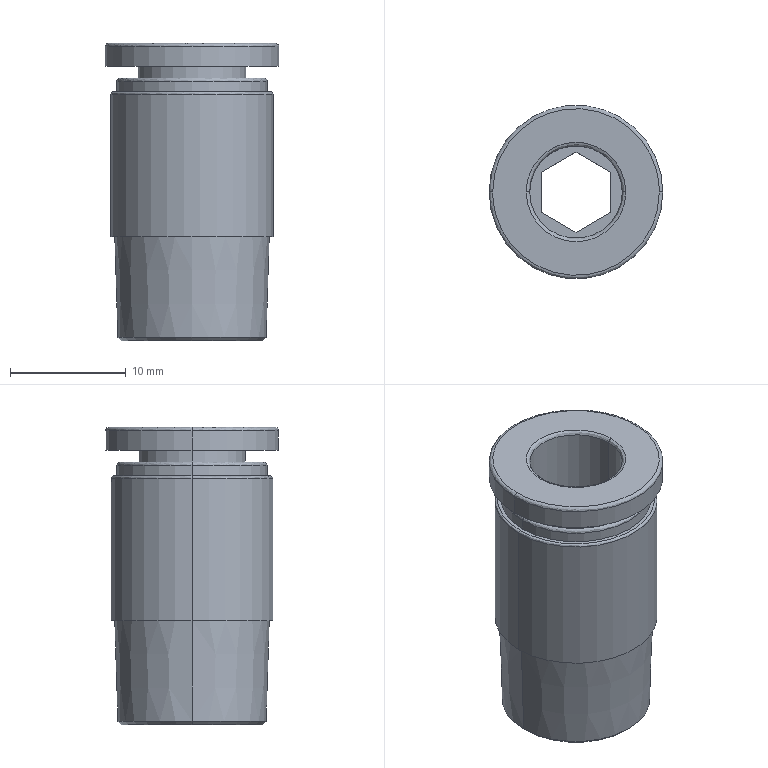Part | STEP file | 1 solid | 40 faces | box 15 x 15 x 25.7 mm | volume 2155 mm3 | plane 14 | cylinder 10 | cone 8 | spline 8 | commonest cylinder face diameters 8 x2 9.3 x2 13 x2 14 x2 15 x2